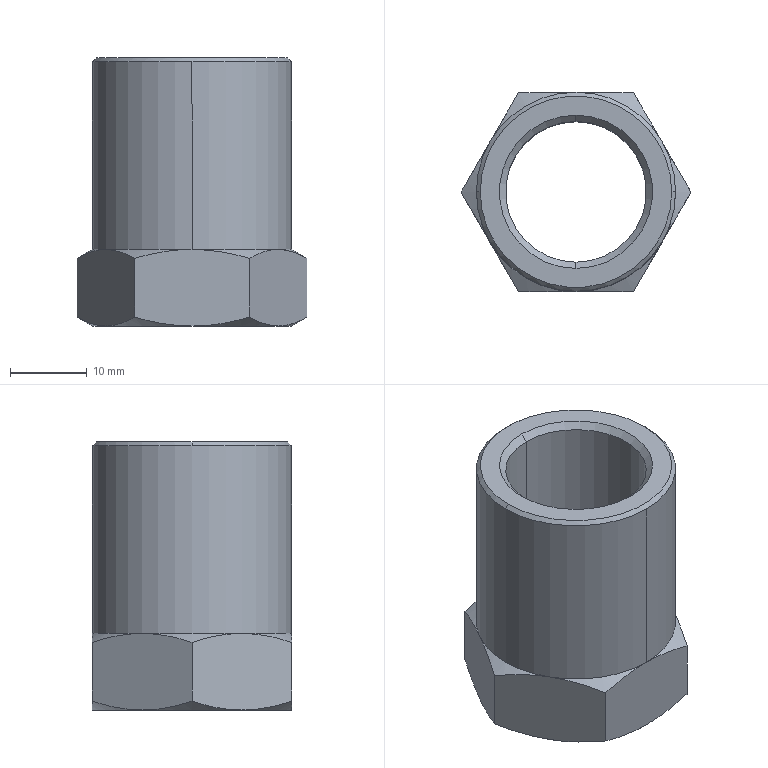Part | STEP file | 1 solid | 31 faces | box 30.022 x 26 x 35 mm | volume 9758 mm3 | cone 19 | plane 8 | cylinder 4 | commonest cylinder face diameters 18.376 x2 26 x2